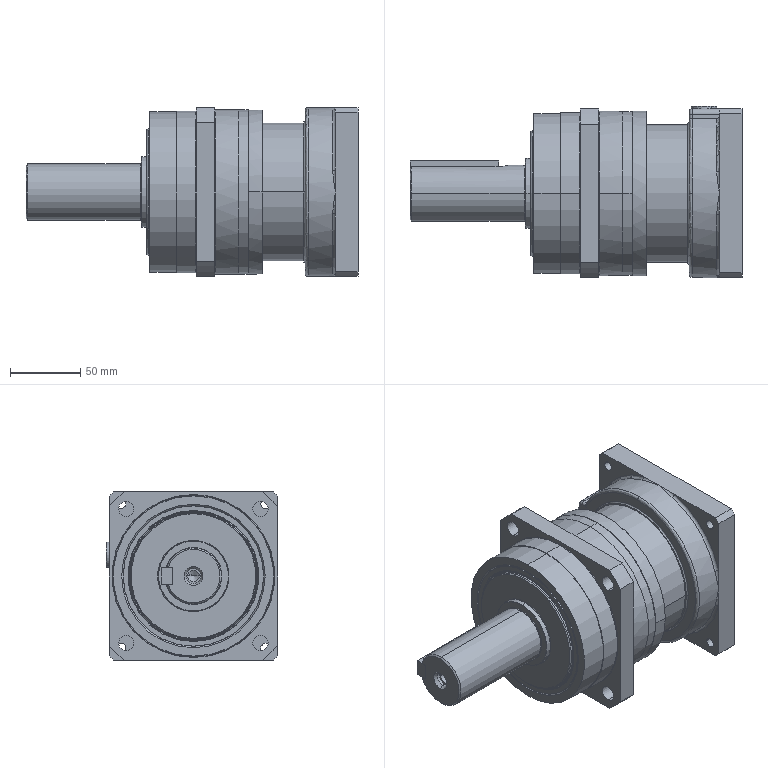Part | STEP file | ANFX-P130W-1SL3-21 | 82 solids | 1141 faces | box 236 x 122 x 120 mm | volume 1055212 mm3 | cylinder 338 | spline 246 | cone 228 | torus 172 | plane 157 | commonest cylinder face diameters 4.5 x36 11 x25 3.242 x24 4.917 x24 6.6 x18 100 x16